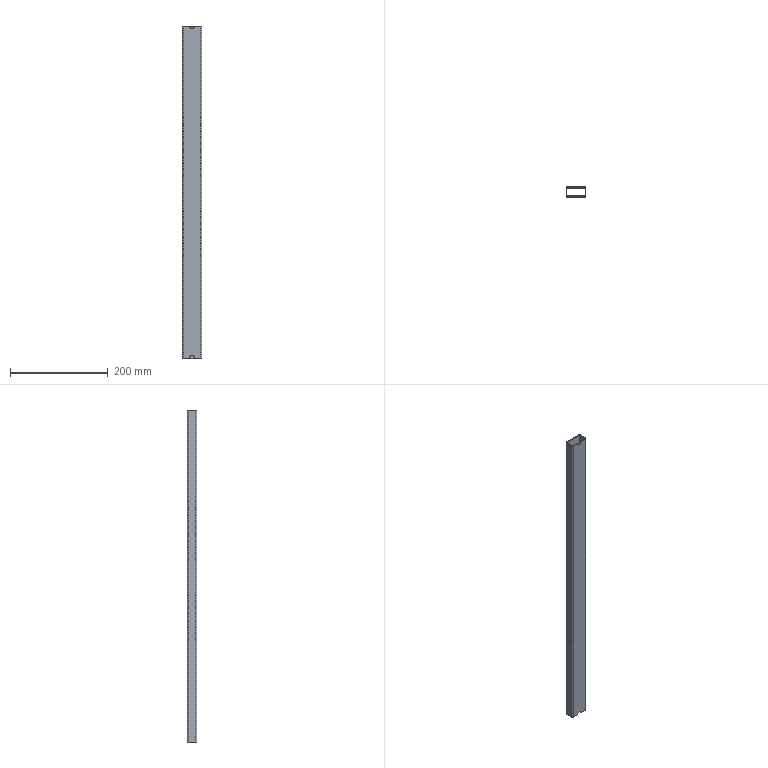Part | STEP file | 6150102 | 1 solid | 20 faces | box 40 x 20 x 680 mm | volume 113098 mm3 | plane 10 | cylinder 10 | commonest cylinder face diameters 2 x4 5 x4 10 x2
STEP:
#1=CARTESIAN_POINT('',(5.,0.,340.));
#2=VERTEX_POINT('',#1);
#3=CARTESIAN_POINT('',(-5.,0.,340.));
#4=VERTEX_POINT('',#3);
#5=CARTESIAN_POINT('',(0.,0.,340.));
#6=DIRECTION('',(0.,1.,0.));
#7=DIRECTION('',(0.,0.,1.));
#8=AXIS2_PLACEMENT_3D('',#5,#6,#7);
#9=CIRCLE('',#8,5.);
#10=EDGE_CURVE('',#2,#4,#9,.T.);
#11=ORIENTED_EDGE('',*,*,#10,.T.);
#12=CARTESIAN_POINT('',(-17.5,0.,340.));
#13=VERTEX_POINT('',#12);
#14=CARTESIAN_POINT('',(17.5,0.,340.));
#15=DIRECTION('',(1.,0.,0.));
#16=VECTOR('',#15,1000.);
#17=LINE('',#14,#16);
#18=EDGE_CURVE('',#13,#4,#17,.T.);
#19=ORIENTED_EDGE('',*,*,#18,.F.);
#20=CARTESIAN_POINT('',(-17.5,0.,-340.));
#21=VERTEX_POINT('',#20);
#22=CARTESIAN_POINT('',(-17.5,0.,340.));
#23=DIRECTION('',(0.,0.,-1.));
#24=VECTOR('',#23,1000.);
#25=LINE('',#22,#24);
#26=EDGE_CURVE('',#13,#21,#25,.T.);
#27=ORIENTED_EDGE('',*,*,#26,.T.);
#28=CARTESIAN_POINT('',(-5.,0.,-340.));
#29=VERTEX_POINT('',#28);
#30=CARTESIAN_POINT('',(17.5,0.,-340.));
#31=DIRECTION('',(1.,0.,0.));
#32=VECTOR('',#31,1000.);
#33=LINE('',#30,#32);
#34=EDGE_CURVE('',#21,#29,#33,.T.);
#35=ORIENTED_EDGE('',*,*,#34,.T.);
#36=CARTESIAN_POINT('',(5.,0.,-340.));
#37=VERTEX_POINT('',#36);
#38=CARTESIAN_POINT('',(0.,0.,-340.));
#39=DIRECTION('',(0.,1.,0.));
#40=DIRECTION('',(0.,0.,1.));
#41=AXIS2_PLACEMENT_3D('',#38,#39,#40);
#42=CIRCLE('',#41,5.);
#43=EDGE_CURVE('',#29,#37,#42,.T.);
#44=ORIENTED_EDGE('',*,*,#43,.T.);
#45=CARTESIAN_POINT('',(17.5,0.,-340.));
#46=VERTEX_POINT('',#45);
#47=CARTESIAN_POINT('',(17.5,0.,-340.));
#48=DIRECTION('',(1.,0.,0.));
#49=VECTOR('',#48,1000.);
#50=LINE('',#47,#49);
#51=EDGE_CURVE('',#37,#46,#50,.T.);
#52=ORIENTED_EDGE('',*,*,#51,.T.);
#53=CARTESIAN_POINT('',(17.5,0.,340.));
#54=VERTEX_POINT('',#53);
#55=CARTESIAN_POINT('',(17.5,0.,340.));
#56=DIRECTION('',(0.,0.,-1.));
#57=VECTOR('',#56,1000.);
#58=LINE('',#55,#57);
#59=EDGE_CURVE('',#54,#46,#58,.T.);
#60=ORIENTED_EDGE('',*,*,#59,.F.);
#61=CARTESIAN_POINT('',(17.5,0.,340.));
#62=DIRECTION('',(1.,0.,0.));
#63=VECTOR('',#62,1000.);
#64=LINE('',#61,#63);
#65=EDGE_CURVE('',#2,#54,#64,.T.);
#66=ORIENTED_EDGE('',*,*,#65,.F.);
#67=EDGE_LOOP('',(#11,#19,#27,#35,#44,#52,#60,#66));
#68=FACE_OUTER_BOUND('',#67,.T.);
#69=CARTESIAN_POINT('',(17.5,0.,340.));
#70=DIRECTION('',(0.,1.,0.));
#71=DIRECTION('',(0.,0.,1.));
#72=AXIS2_PLACEMENT_3D('',#69,#70,#71);
#73=PLANE('',#72);
#74=ADVANCED_FACE('',(#68),#73,.F.);
#75=CARTESIAN_POINT('',(-17.5,1.5,340.));
#76=VERTEX_POINT('',#75);
#77=CARTESIAN_POINT('',(-5.,1.5,340.));
#78=VERTEX_POINT('',#77);
#79=CARTESIAN_POINT('',(17.5,1.5,340.));
#80=DIRECTION('',(1.,0.,0.));
#81=VECTOR('',#80,1000.);
#82=LINE('',#79,#81);
#83=EDGE_CURVE('',#76,#78,#82,.T.);
#84=ORIENTED_EDGE('',*,*,#83,.T.);
#85=CARTESIAN_POINT('',(5.,1.5,340.));
#86=VERTEX_POINT('',#85);
#87=CARTESIAN_POINT('',(0.,1.5,340.));
#88=DIRECTION('',(0.,-1.,0.));
#89=DIRECTION('',(-1.,0.,0.));
#90=AXIS2_PLACEMENT_3D('',#87,#88,#89);
#91=CIRCLE('',#90,5.);
#92=EDGE_CURVE('',#78,#86,#91,.T.);
#93=ORIENTED_EDGE('',*,*,#92,.T.);
#94=CARTESIAN_POINT('',(17.5,1.5,340.));
#95=VERTEX_POINT('',#94);
#96=CARTESIAN_POINT('',(17.5,1.5,340.));
#97=DIRECTION('',(1.,0.,0.));
#98=VECTOR('',#97,1000.);
#99=LINE('',#96,#98);
#100=EDGE_CURVE('',#86,#95,#99,.T.);
#101=ORIENTED_EDGE('',*,*,#100,.T.);
#102=CARTESIAN_POINT('',(17.5,1.5,-340.));
#103=VERTEX_POINT('',#102);
#104=CARTESIAN_POINT('',(17.5,1.5,340.));
#105=DIRECTION('',(0.,0.,-1.));
#106=VECTOR('',#105,1000.);
#107=LINE('',#104,#106);
#108=EDGE_CURVE('',#95,#103,#107,.T.);
#109=ORIENTED_EDGE('',*,*,#108,.T.);
#110=CARTESIAN_POINT('',(5.,1.5,-340.));
#111=VERTEX_POINT('',#110);
#112=CARTESIAN_POINT('',(17.5,1.5,-340.));
#113=DIRECTION('',(1.,0.,0.));
#114=VECTOR('',#113,1000.);
#115=LINE('',#112,#114);
#116=EDGE_CURVE('',#111,#103,#115,.T.);
#117=ORIENTED_EDGE('',*,*,#116,.F.);
#118=CARTESIAN_POINT('',(-5.,1.5,-340.));
#119=VERTEX_POINT('',#118);
#120=CARTESIAN_POINT('',(0.,1.5,-340.));
#121=DIRECTION('',(0.,-1.,0.));
#122=DIRECTION('',(-1.,0.,0.));
#123=AXIS2_PLACEMENT_3D('',#120,#121,#122);
#124=CIRCLE('',#123,5.);
#125=EDGE_CURVE('',#111,#119,#124,.T.);
#126=ORIENTED_EDGE('',*,*,#125,.T.);
#127=CARTESIAN_POINT('',(-17.5,1.5,-340.));
#128=VERTEX_POINT('',#127);
#129=CARTESIAN_POINT('',(17.5,1.5,-340.));
#130=DIRECTION('',(1.,0.,0.));
#131=VECTOR('',#130,1000.);
#132=LINE('',#129,#131);
#133=EDGE_CURVE('',#128,#119,#132,.T.);
#134=ORIENTED_EDGE('',*,*,#133,.F.);
#135=CARTESIAN_POINT('',(-17.5,1.5,340.));
#136=DIRECTION('',(0.,0.,-1.));
#137=VECTOR('',#136,1000.);
#138=LINE('',#135,#137);
#139=EDGE_CURVE('',#76,#128,#138,.T.);
#140=ORIENTED_EDGE('',*,*,#139,.F.);
#141=EDGE_LOOP('',(#84,#93,#101,#109,#117,#126,#134,#140));
#142=FACE_OUTER_BOUND('',#141,.T.);
#143=CARTESIAN_POINT('',(17.5,1.5,340.));
#144=DIRECTION('',(0.,1.,0.));
#145=DIRECTION('',(-1.,0.,0.));
#146=AXIS2_PLACEMENT_3D('',#143,#144,#145);
#147=PLANE('',#146);
#148=ADVANCED_FACE('',(#142),#147,.T.);
#149=CARTESIAN_POINT('',(5.,10.,340.));
#150=DIRECTION('',(0.,1.,0.));
#151=VECTOR('',#150,1000.);
#152=LINE('',#149,#151);
#153=EDGE_CURVE('',#2,#86,#152,.T.);
#154=ORIENTED_EDGE('',*,*,#153,.F.);
#155=ORIENTED_EDGE('',*,*,#65,.T.);
#156=CARTESIAN_POINT('',(20.,2.5,340.));
#157=VERTEX_POINT('',#156);
#158=CARTESIAN_POINT('',(17.5,2.5,340.));
#159=DIRECTION('',(0.,0.,1.));
#160=DIRECTION('',(-1.,0.,0.));
#161=AXIS2_PLACEMENT_3D('',#158,#159,#160);
#162=CIRCLE('',#161,2.5);
#163=EDGE_CURVE('',#54,#157,#162,.T.);
#164=ORIENTED_EDGE('',*,*,#163,.T.);
#165=CARTESIAN_POINT('',(20.,17.5,340.));
#166=VERTEX_POINT('',#165);
#167=CARTESIAN_POINT('',(20.,2.5,340.));
#168=DIRECTION('',(0.,1.,0.));
#169=VECTOR('',#168,1000.);
#170=LINE('',#167,#169);
#171=EDGE_CURVE('',#157,#166,#170,.T.);
#172=ORIENTED_EDGE('',*,*,#171,.T.);
#173=CARTESIAN_POINT('',(17.5,20.,340.));
#174=VERTEX_POINT('',#173);
#175=CARTESIAN_POINT('',(17.5,17.5,340.));
#176=DIRECTION('',(0.,0.,1.));
#177=DIRECTION('',(-1.,0.,0.));
#178=AXIS2_PLACEMENT_3D('',#175,#176,#177);
#179=CIRCLE('',#178,2.5);
#180=EDGE_CURVE('',#166,#174,#179,.T.);
#181=ORIENTED_EDGE('',*,*,#180,.T.);
#182=CARTESIAN_POINT('',(-17.5,20.,340.));
#183=VERTEX_POINT('',#182);
#184=CARTESIAN_POINT('',(17.5,20.,340.));
#185=DIRECTION('',(-1.,0.,0.));
#186=VECTOR('',#185,1000.);
#187=LINE('',#184,#186);
#188=EDGE_CURVE('',#174,#183,#187,.T.);
#189=ORIENTED_EDGE('',*,*,#188,.T.);
#190=CARTESIAN_POINT('',(-20.,17.5,340.));
#191=VERTEX_POINT('',#190);
#192=CARTESIAN_POINT('',(-17.5,17.5,340.));
#193=DIRECTION('',(0.,0.,1.));
#194=DIRECTION('',(-1.,0.,0.));
#195=AXIS2_PLACEMENT_3D('',#192,#193,#194);
#196=CIRCLE('',#195,2.5);
#197=EDGE_CURVE('',#183,#191,#196,.T.);
#198=ORIENTED_EDGE('',*,*,#197,.T.);
#199=CARTESIAN_POINT('',(-20.,2.5,340.));
#200=VERTEX_POINT('',#199);
#201=CARTESIAN_POINT('',(-20.,2.5,340.));
#202=DIRECTION('',(0.,-1.,0.));
#203=VECTOR('',#202,1000.);
#204=LINE('',#201,#203);
#205=EDGE_CURVE('',#191,#200,#204,.T.);
#206=ORIENTED_EDGE('',*,*,#205,.T.);
#207=CARTESIAN_POINT('',(-17.5,2.5,340.));
#208=DIRECTION('',(0.,0.,1.));
#209=DIRECTION('',(-1.,0.,0.));
#210=AXIS2_PLACEMENT_3D('',#207,#208,#209);
#211=CIRCLE('',#210,2.5);
#212=EDGE_CURVE('',#200,#13,#211,.T.);
#213=ORIENTED_EDGE('',*,*,#212,.T.);
#214=ORIENTED_EDGE('',*,*,#18,.T.);
#215=CARTESIAN_POINT('',(-5.,10.,340.));
#216=DIRECTION('',(0.,-1.,0.));
#217=VECTOR('',#216,1000.);
#218=LINE('',#215,#217);
#219=EDGE_CURVE('',#78,#4,#218,.T.);
#220=ORIENTED_EDGE('',*,*,#219,.F.);
#221=ORIENTED_EDGE('',*,*,#83,.F.);
#222=CARTESIAN_POINT('',(-18.5,2.5,340.));
#223=VERTEX_POINT('',#222);
#224=CARTESIAN_POINT('',(-17.5,2.5,340.));
#225=DIRECTION('',(0.,0.,1.));
#226=DIRECTION('',(-1.,0.,0.));
#227=AXIS2_PLACEMENT_3D('',#224,#225,#226);
#228=CIRCLE('',#227,1.);
#229=EDGE_CURVE('',#223,#76,#228,.T.);
#230=ORIENTED_EDGE('',*,*,#229,.F.);
#231=CARTESIAN_POINT('',(-18.5,17.5,340.));
#232=VERTEX_POINT('',#231);
#233=CARTESIAN_POINT('',(-18.5,2.5,340.));
#234=DIRECTION('',(0.,-1.,0.));
#235=VECTOR('',#234,1000.);
#236=LINE('',#233,#235);
#237=EDGE_CURVE('',#232,#223,#236,.T.);
#238=ORIENTED_EDGE('',*,*,#237,.F.);
#239=CARTESIAN_POINT('',(-17.5,18.5,340.));
#240=VERTEX_POINT('',#239);
#241=CARTESIAN_POINT('',(-17.5,17.5,340.));
#242=DIRECTION('',(0.,0.,1.));
#243=DIRECTION('',(-1.,0.,0.));
#244=AXIS2_PLACEMENT_3D('',#241,#242,#243);
#245=CIRCLE('',#244,1.);
#246=EDGE_CURVE('',#240,#232,#245,.T.);
#247=ORIENTED_EDGE('',*,*,#246,.F.);
#248=CARTESIAN_POINT('',(17.5,18.5,340.));
#249=VERTEX_POINT('',#248);
#250=CARTESIAN_POINT('',(17.5,18.5,340.));
#251=DIRECTION('',(-1.,0.,0.));
#252=VECTOR('',#251,1000.);
#253=LINE('',#250,#252);
#254=EDGE_CURVE('',#249,#240,#253,.T.);
#255=ORIENTED_EDGE('',*,*,#254,.F.);
#256=CARTESIAN_POINT('',(18.5,17.5,340.));
#257=VERTEX_POINT('',#256);
#258=CARTESIAN_POINT('',(17.5,17.5,340.));
#259=DIRECTION('',(0.,0.,1.));
#260=DIRECTION('',(-1.,0.,0.));
#261=AXIS2_PLACEMENT_3D('',#258,#259,#260);
#262=CIRCLE('',#261,1.);
#263=EDGE_CURVE('',#257,#249,#262,.T.);
#264=ORIENTED_EDGE('',*,*,#263,.F.);
#265=CARTESIAN_POINT('',(18.5,2.5,340.));
#266=VERTEX_POINT('',#265);
#267=CARTESIAN_POINT('',(18.5,2.5,340.));
#268=DIRECTION('',(0.,1.,0.));
#269=VECTOR('',#268,1000.);
#270=LINE('',#267,#269);
#271=EDGE_CURVE('',#266,#257,#270,.T.);
#272=ORIENTED_EDGE('',*,*,#271,.F.);
#273=CARTESIAN_POINT('',(17.5,2.5,340.));
#274=DIRECTION('',(0.,0.,1.));
#275=DIRECTION('',(-1.,0.,0.));
#276=AXIS2_PLACEMENT_3D('',#273,#274,#275);
#277=CIRCLE('',#276,1.);
#278=EDGE_CURVE('',#95,#266,#277,.T.);
#279=ORIENTED_EDGE('',*,*,#278,.F.);
#280=ORIENTED_EDGE('',*,*,#100,.F.);
#281=EDGE_LOOP('',(#154,#155,#164,#172,#181,#189,#198,#206,#213,#214,#220,#221,#230,#238,#247,#255,#264,#272,#279,#280));
#282=FACE_OUTER_BOUND('',#281,.T.);
#283=CARTESIAN_POINT('',(-17.5,17.5,340.));
#284=DIRECTION('',(0.,0.,-1.));
#285=DIRECTION('',(-1.,0.,0.));
#286=AXIS2_PLACEMENT_3D('',#283,#284,#285);
#287=PLANE('',#286);
#288=ADVANCED_FACE('',(#282),#287,.F.);
#289=ORIENTED_EDGE('',*,*,#51,.F.);
#290=CARTESIAN_POINT('',(5.,10.,-340.));
#291=DIRECTION('',(0.,1.,0.));
#292=VECTOR('',#291,1000.);
#293=LINE('',#290,#292);
#294=EDGE_CURVE('',#37,#111,#293,.T.);
#295=ORIENTED_EDGE('',*,*,#294,.T.);
#296=ORIENTED_EDGE('',*,*,#116,.T.);
#297=CARTESIAN_POINT('',(18.5,2.5,-340.));
#298=VERTEX_POINT('',#297);
#299=CARTESIAN_POINT('',(17.5,2.5,-340.));
#300=DIRECTION('',(0.,0.,1.));
#301=DIRECTION('',(-1.,0.,0.));
#302=AXIS2_PLACEMENT_3D('',#299,#300,#301);
#303=CIRCLE('',#302,1.);
#304=EDGE_CURVE('',#103,#298,#303,.T.);
#305=ORIENTED_EDGE('',*,*,#304,.T.);
#306=CARTESIAN_POINT('',(18.5,17.5,-340.));
#307=VERTEX_POINT('',#306);
#308=CARTESIAN_POINT('',(18.5,2.5,-340.));
#309=DIRECTION('',(0.,1.,0.));
#310=VECTOR('',#309,1000.);
#311=LINE('',#308,#310);
#312=EDGE_CURVE('',#298,#307,#311,.T.);
#313=ORIENTED_EDGE('',*,*,#312,.T.);
#314=CARTESIAN_POINT('',(17.5,18.5,-340.));
#315=VERTEX_POINT('',#314);
#316=CARTESIAN_POINT('',(17.5,17.5,-340.));
#317=DIRECTION('',(0.,0.,1.));
#318=DIRECTION('',(-1.,0.,0.));
#319=AXIS2_PLACEMENT_3D('',#316,#317,#318);
#320=CIRCLE('',#319,1.);
#321=EDGE_CURVE('',#307,#315,#320,.T.);
#322=ORIENTED_EDGE('',*,*,#321,.T.);
#323=CARTESIAN_POINT('',(-17.5,18.5,-340.));
#324=VERTEX_POINT('',#323);
#325=CARTESIAN_POINT('',(17.5,18.5,-340.));
#326=DIRECTION('',(-1.,0.,0.));
#327=VECTOR('',#326,1000.);
#328=LINE('',#325,#327);
#329=EDGE_CURVE('',#315,#324,#328,.T.);
#330=ORIENTED_EDGE('',*,*,#329,.T.);
#331=CARTESIAN_POINT('',(-18.5,17.5,-340.));
#332=VERTEX_POINT('',#331);
#333=CARTESIAN_POINT('',(-17.5,17.5,-340.));
#334=DIRECTION('',(0.,0.,1.));
#335=DIRECTION('',(-1.,0.,0.));
#336=AXIS2_PLACEMENT_3D('',#333,#334,#335);
#337=CIRCLE('',#336,1.);
#338=EDGE_CURVE('',#324,#332,#337,.T.);
#339=ORIENTED_EDGE('',*,*,#338,.T.);
#340=CARTESIAN_POINT('',(-18.5,2.5,-340.));
#341=VERTEX_POINT('',#340);
#342=CARTESIAN_POINT('',(-18.5,2.5,-340.));
#343=DIRECTION('',(0.,-1.,0.));
#344=VECTOR('',#343,1000.);
#345=LINE('',#342,#344);
#346=EDGE_CURVE('',#332,#341,#345,.T.);
#347=ORIENTED_EDGE('',*,*,#346,.T.);
#348=CARTESIAN_POINT('',(-17.5,2.5,-340.));
#349=DIRECTION('',(0.,0.,1.));
#350=DIRECTION('',(-1.,0.,0.));
#351=AXIS2_PLACEMENT_3D('',#348,#349,#350);
#352=CIRCLE('',#351,1.);
#353=EDGE_CURVE('',#341,#128,#352,.T.);
#354=ORIENTED_EDGE('',*,*,#353,.T.);
#355=ORIENTED_EDGE('',*,*,#133,.T.);
#356=CARTESIAN_POINT('',(-5.,10.,-340.));
#357=DIRECTION('',(0.,-1.,0.));
#358=VECTOR('',#357,1000.);
#359=LINE('',#356,#358);
#360=EDGE_CURVE('',#119,#29,#359,.T.);
#361=ORIENTED_EDGE('',*,*,#360,.T.);
#362=ORIENTED_EDGE('',*,*,#34,.F.);
#363=CARTESIAN_POINT('',(-20.,2.5,-340.));
#364=VERTEX_POINT('',#363);
#365=CARTESIAN_POINT('',(-17.5,2.5,-340.));
#366=DIRECTION('',(0.,0.,1.));
#367=DIRECTION('',(-1.,0.,0.));
#368=AXIS2_PLACEMENT_3D('',#365,#366,#367);
#369=CIRCLE('',#368,2.5);
#370=EDGE_CURVE('',#364,#21,#369,.T.);
#371=ORIENTED_EDGE('',*,*,#370,.F.);
#372=CARTESIAN_POINT('',(-20.,17.5,-340.));
#373=VERTEX_POINT('',#372);
#374=CARTESIAN_POINT('',(-20.,2.5,-340.));
#375=DIRECTION('',(0.,-1.,0.));
#376=VECTOR('',#375,1000.);
#377=LINE('',#374,#376);
#378=EDGE_CURVE('',#373,#364,#377,.T.);
#379=ORIENTED_EDGE('',*,*,#378,.F.);
#380=CARTESIAN_POINT('',(-17.5,20.,-340.));
#381=VERTEX_POINT('',#380);
#382=CARTESIAN_POINT('',(-17.5,17.5,-340.));
#383=DIRECTION('',(0.,0.,1.));
#384=DIRECTION('',(-1.,0.,0.));
#385=AXIS2_PLACEMENT_3D('',#382,#383,#384);
#386=CIRCLE('',#385,2.5);
#387=EDGE_CURVE('',#381,#373,#386,.T.);
#388=ORIENTED_EDGE('',*,*,#387,.F.);
#389=CARTESIAN_POINT('',(17.5,20.,-340.));
#390=VERTEX_POINT('',#389);
#391=CARTESIAN_POINT('',(17.5,20.,-340.));
#392=DIRECTION('',(-1.,0.,0.));
#393=VECTOR('',#392,1000.);
#394=LINE('',#391,#393);
#395=EDGE_CURVE('',#390,#381,#394,.T.);
#396=ORIENTED_EDGE('',*,*,#395,.F.);
#397=CARTESIAN_POINT('',(20.,17.5,-340.));
#398=VERTEX_POINT('',#397);
#399=CARTESIAN_POINT('',(17.5,17.5,-340.));
#400=DIRECTION('',(0.,0.,1.));
#401=DIRECTION('',(-1.,0.,0.));
#402=AXIS2_PLACEMENT_3D('',#399,#400,#401);
#403=CIRCLE('',#402,2.5);
#404=EDGE_CURVE('',#398,#390,#403,.T.);
#405=ORIENTED_EDGE('',*,*,#404,.F.);
#406=CARTESIAN_POINT('',(20.,2.5,-340.));
#407=VERTEX_POINT('',#406);
#408=CARTESIAN_POINT('',(20.,2.5,-340.));
#409=DIRECTION('',(0.,1.,0.));
#410=VECTOR('',#409,1000.);
#411=LINE('',#408,#410);
#412=EDGE_CURVE('',#407,#398,#411,.T.);
#413=ORIENTED_EDGE('',*,*,#412,.F.);
#414=CARTESIAN_POINT('',(17.5,2.5,-340.));
#415=DIRECTION('',(0.,0.,1.));
#416=DIRECTION('',(-1.,0.,0.));
#417=AXIS2_PLACEMENT_3D('',#414,#415,#416);
#418=CIRCLE('',#417,2.5);
#419=EDGE_CURVE('',#46,#407,#418,.T.);
#420=ORIENTED_EDGE('',*,*,#419,.F.);
#421=EDGE_LOOP('',(#289,#295,#296,#305,#313,#322,#330,#339,#347,#354,#355,#361,#362,#371,#379,#388,#396,#405,#413,#420));
#422=FACE_OUTER_BOUND('',#421,.T.);
#423=CARTESIAN_POINT('',(-17.5,17.5,-340.));
#424=DIRECTION('',(0.,0.,-1.));
#425=DIRECTION('',(-1.,0.,0.));
#426=AXIS2_PLACEMENT_3D('',#423,#424,#425);
#427=PLANE('',#426);
#428=ADVANCED_FACE('',(#422),#427,.T.);
#429=ORIENTED_EDGE('',*,*,#387,.T.);
#430=CARTESIAN_POINT('',(-20.,17.5,340.));
#431=DIRECTION('',(0.,0.,-1.));
#432=VECTOR('',#431,1000.);
#433=LINE('',#430,#432);
#434=EDGE_CURVE('',#191,#373,#433,.T.);
#435=ORIENTED_EDGE('',*,*,#434,.F.);
#436=ORIENTED_EDGE('',*,*,#197,.F.);
#437=CARTESIAN_POINT('',(-17.5,20.,340.));
#438=DIRECTION('',(0.,0.,-1.));
#439=VECTOR('',#438,1000.);
#440=LINE('',#437,#439);
#441=EDGE_CURVE('',#183,#381,#440,.T.);
#442=ORIENTED_EDGE('',*,*,#441,.T.);
#443=EDGE_LOOP('',(#429,#435,#436,#442));
#444=FACE_OUTER_BOUND('',#443,.T.);
#445=CARTESIAN_POINT('',(-17.5,17.5,340.));
#446=DIRECTION('',(0.,0.,-1.));
#447=DIRECTION('',(-1.,0.,0.));
#448=AXIS2_PLACEMENT_3D('',#445,#446,#447);
#449=CYLINDRICAL_SURFACE('',#448,2.5);
#450=ADVANCED_FACE('',(#444),#449,.T.);
#451=ORIENTED_EDGE('',*,*,#378,.T.);
#452=CARTESIAN_POINT('',(-20.,2.5,340.));
#453=DIRECTION('',(0.,0.,-1.));
#454=VECTOR('',#453,1000.);
#455=LINE('',#452,#454);
#456=EDGE_CURVE('',#200,#364,#455,.T.);
#457=ORIENTED_EDGE('',*,*,#456,.F.);
#458=ORIENTED_EDGE('',*,*,#205,.F.);
#459=ORIENTED_EDGE('',*,*,#434,.T.);
#460=EDGE_LOOP('',(#451,#457,#458,#459));
#461=FACE_OUTER_BOUND('',#460,.T.);
#462=CARTESIAN_POINT('',(-20.,2.5,340.));
#463=DIRECTION('',(1.,0.,0.));
#464=DIRECTION('',(0.,1.,0.));
#465=AXIS2_PLACEMENT_3D('',#462,#463,#464);
#466=PLANE('',#465);
#467=ADVANCED_FACE('',(#461),#466,.F.);
#468=ORIENTED_EDGE('',*,*,#370,.T.);
#469=ORIENTED_EDGE('',*,*,#26,.F.);
#470=ORIENTED_EDGE('',*,*,#212,.F.);
#471=ORIENTED_EDGE('',*,*,#456,.T.);
#472=EDGE_LOOP('',(#468,#469,#470,#471));
#473=FACE_OUTER_BOUND('',#472,.T.);
#474=CARTESIAN_POINT('',(-17.5,2.5,340.));
#475=DIRECTION('',(0.,0.,-1.));
#476=DIRECTION('',(-1.,0.,0.));
#477=AXIS2_PLACEMENT_3D('',#474,#475,#476);
#478=CYLINDRICAL_SURFACE('',#477,2.5);
#479=ADVANCED_FACE('',(#473),#478,.T.);
#480=ORIENTED_EDGE('',*,*,#419,.T.);
#481=CARTESIAN_POINT('',(20.,2.5,340.));
#482=DIRECTION('',(0.,0.,-1.));
#483=VECTOR('',#482,1000.);
#484=LINE('',#481,#483);
#485=EDGE_CURVE('',#157,#407,#484,.T.);
#486=ORIENTED_EDGE('',*,*,#485,.F.);
#487=ORIENTED_EDGE('',*,*,#163,.F.);
#488=ORIENTED_EDGE('',*,*,#59,.T.);
#489=EDGE_LOOP('',(#480,#486,#487,#488));
#490=FACE_OUTER_BOUND('',#489,.T.);
#491=CARTESIAN_POINT('',(17.5,2.5,340.));
#492=DIRECTION('',(0.,0.,-1.));
#493=DIRECTION('',(-1.,0.,0.));
#494=AXIS2_PLACEMENT_3D('',#491,#492,#493);
#495=CYLINDRICAL_SURFACE('',#494,2.5);
#496=ADVANCED_FACE('',(#490),#495,.T.);
#497=ORIENTED_EDGE('',*,*,#412,.T.);
#498=CARTESIAN_POINT('',(20.,17.5,340.));
#499=DIRECTION('',(0.,0.,-1.));
#500=VECTOR('',#499,1000.);
#501=LINE('',#498,#500);
#502=EDGE_CURVE('',#166,#398,#501,.T.);
#503=ORIENTED_EDGE('',*,*,#502,.F.);
#504=ORIENTED_EDGE('',*,*,#171,.F.);
#505=ORIENTED_EDGE('',*,*,#485,.T.);
#506=EDGE_LOOP('',(#497,#503,#504,#505));
#507=FACE_OUTER_BOUND('',#506,.T.);
#508=CARTESIAN_POINT('',(20.,2.5,340.));
#509=DIRECTION('',(-1.,0.,0.));
#510=DIRECTION('',(0.,-1.,0.));
#511=AXIS2_PLACEMENT_3D('',#508,#509,#510);
#512=PLANE('',#511);
#513=ADVANCED_FACE('',(#507),#512,.F.);
#514=ORIENTED_EDGE('',*,*,#404,.T.);
#515=CARTESIAN_POINT('',(17.5,20.,340.));
#516=DIRECTION('',(0.,0.,-1.));
#517=VECTOR('',#516,1000.);
#518=LINE('',#515,#517);
#519=EDGE_CURVE('',#174,#390,#518,.T.);
#520=ORIENTED_EDGE('',*,*,#519,.F.);
#521=ORIENTED_EDGE('',*,*,#180,.F.);
#522=ORIENTED_EDGE('',*,*,#502,.T.);
#523=EDGE_LOOP('',(#514,#520,#521,#522));
#524=FACE_OUTER_BOUND('',#523,.T.);
#525=CARTESIAN_POINT('',(17.5,17.5,340.));
#526=DIRECTION('',(0.,0.,-1.));
#527=DIRECTION('',(-1.,0.,0.));
#528=AXIS2_PLACEMENT_3D('',#525,#526,#527);
#529=CYLINDRICAL_SURFACE('',#528,2.5);
#530=ADVANCED_FACE('',(#524),#529,.T.);
#531=ORIENTED_EDGE('',*,*,#395,.T.);
#532=ORIENTED_EDGE('',*,*,#441,.F.);
#533=ORIENTED_EDGE('',*,*,#188,.F.);
#534=ORIENTED_EDGE('',*,*,#519,.T.);
#535=EDGE_LOOP('',(#531,#532,#533,#534));
#536=FACE_OUTER_BOUND('',#535,.T.);
#537=CARTESIAN_POINT('',(17.5,20.,340.));
#538=DIRECTION('',(0.,-1.,0.));
#539=DIRECTION('',(0.,0.,-1.));
#540=AXIS2_PLACEMENT_3D('',#537,#538,#539);
#541=PLANE('',#540);
#542=ADVANCED_FACE('',(#536),#541,.F.);
#543=ORIENTED_EDGE('',*,*,#304,.F.);
#544=ORIENTED_EDGE('',*,*,#108,.F.);
#545=ORIENTED_EDGE('',*,*,#278,.T.);
#546=CARTESIAN_POINT('',(18.5,2.5,340.));
#547=DIRECTION('',(0.,0.,-1.));
#548=VECTOR('',#547,1000.);
#549=LINE('',#546,#548);
#550=EDGE_CURVE('',#266,#298,#549,.T.);
#551=ORIENTED_EDGE('',*,*,#550,.T.);
#552=EDGE_LOOP('',(#543,#544,#545,#551));
#553=FACE_OUTER_BOUND('',#552,.T.);
#554=CARTESIAN_POINT('',(17.5,2.5,340.));
#555=DIRECTION('',(0.,0.,-1.));
#556=DIRECTION('',(-1.,0.,0.));
#557=AXIS2_PLACEMENT_3D('',#554,#555,#556);
#558=CYLINDRICAL_SURFACE('',#557,1.);
#559=ADVANCED_FACE('',(#553),#558,.F.);
#560=ORIENTED_EDGE('',*,*,#312,.F.);
#561=ORIENTED_EDGE('',*,*,#550,.F.);
#562=ORIENTED_EDGE('',*,*,#271,.T.);
#563=CARTESIAN_POINT('',(18.5,17.5,340.));
#564=DIRECTION('',(0.,0.,-1.));
#565=VECTOR('',#564,1000.);
#566=LINE('',#563,#565);
#567=EDGE_CURVE('',#257,#307,#566,.T.);
#568=ORIENTED_EDGE('',*,*,#567,.T.);
#569=EDGE_LOOP('',(#560,#561,#562,#568));
#570=FACE_OUTER_BOUND('',#569,.T.);
#571=CARTESIAN_POINT('',(18.5,2.5,340.));
#572=DIRECTION('',(-1.,0.,0.));
#573=DIRECTION('',(0.,-1.,0.));
#574=AXIS2_PLACEMENT_3D('',#571,#572,#573);
#575=PLANE('',#574);
#576=ADVANCED_FACE('',(#570),#575,.T.);
#577=ORIENTED_EDGE('',*,*,#321,.F.);
#578=ORIENTED_EDGE('',*,*,#567,.F.);
#579=ORIENTED_EDGE('',*,*,#263,.T.);
#580=CARTESIAN_POINT('',(17.5,18.5,340.));
#581=DIRECTION('',(0.,0.,-1.));
#582=VECTOR('',#581,1000.);
#583=LINE('',#580,#582);
#584=EDGE_CURVE('',#249,#315,#583,.T.);
#585=ORIENTED_EDGE('',*,*,#584,.T.);
#586=EDGE_LOOP('',(#577,#578,#579,#585));
#587=FACE_OUTER_BOUND('',#586,.T.);
#588=CARTESIAN_POINT('',(17.5,17.5,340.));
#589=DIRECTION('',(0.,0.,-1.));
#590=DIRECTION('',(-1.,0.,0.));
#591=AXIS2_PLACEMENT_3D('',#588,#589,#590);
#592=CYLINDRICAL_SURFACE('',#591,1.);
#593=ADVANCED_FACE('',(#587),#592,.F.);
#594=ORIENTED_EDGE('',*,*,#329,.F.);
#595=ORIENTED_EDGE('',*,*,#584,.F.);
#596=ORIENTED_EDGE('',*,*,#254,.T.);
#597=CARTESIAN_POINT('',(-17.5,18.5,340.));
#598=DIRECTION('',(0.,0.,-1.));
#599=VECTOR('',#598,1000.);
#600=LINE('',#597,#599);
#601=EDGE_CURVE('',#240,#324,#600,.T.);
#602=ORIENTED_EDGE('',*,*,#601,.T.);
#603=EDGE_LOOP('',(#594,#595,#596,#602));
#604=FACE_OUTER_BOUND('',#603,.T.);
#605=CARTESIAN_POINT('',(17.5,18.5,340.));
#606=DIRECTION('',(0.,-1.,0.));
#607=DIRECTION('',(0.,0.,-1.));
#608=AXIS2_PLACEMENT_3D('',#605,#606,#607);
#609=PLANE('',#608);
#610=ADVANCED_FACE('',(#604),#609,.T.);
#611=ORIENTED_EDGE('',*,*,#338,.F.);
#612=ORIENTED_EDGE('',*,*,#601,.F.);
#613=ORIENTED_EDGE('',*,*,#246,.T.);
#614=CARTESIAN_POINT('',(-18.5,17.5,340.));
#615=DIRECTION('',(0.,0.,-1.));
#616=VECTOR('',#615,1000.);
#617=LINE('',#614,#616);
#618=EDGE_CURVE('',#232,#332,#617,.T.);
#619=ORIENTED_EDGE('',*,*,#618,.T.);
#620=EDGE_LOOP('',(#611,#612,#613,#619));
#621=FACE_OUTER_BOUND('',#620,.T.);
#622=CARTESIAN_POINT('',(-17.5,17.5,340.));
#623=DIRECTION('',(0.,0.,-1.));
#624=DIRECTION('',(-1.,0.,0.));
#625=AXIS2_PLACEMENT_3D('',#622,#623,#624);
#626=CYLINDRICAL_SURFACE('',#625,1.);
#627=ADVANCED_FACE('',(#621),#626,.F.);
#628=ORIENTED_EDGE('',*,*,#346,.F.);
#629=ORIENTED_EDGE('',*,*,#618,.F.);
#630=ORIENTED_EDGE('',*,*,#237,.T.);
#631=CARTESIAN_POINT('',(-18.5,2.5,340.));
#632=DIRECTION('',(0.,0.,-1.));
#633=VECTOR('',#632,1000.);
#634=LINE('',#631,#633);
#635=EDGE_CURVE('',#223,#341,#634,.T.);
#636=ORIENTED_EDGE('',*,*,#635,.T.);
#637=EDGE_LOOP('',(#628,#629,#630,#636));
#638=FACE_OUTER_BOUND('',#637,.T.);
#639=CARTESIAN_POINT('',(-18.5,2.5,340.));
#640=DIRECTION('',(1.,0.,0.));
#641=DIRECTION('',(0.,1.,0.));
#642=AXIS2_PLACEMENT_3D('',#639,#640,#641);
#643=PLANE('',#642);
#644=ADVANCED_FACE('',(#638),#643,.T.);
#645=ORIENTED_EDGE('',*,*,#353,.F.);
#646=ORIENTED_EDGE('',*,*,#635,.F.);
#647=ORIENTED_EDGE('',*,*,#229,.T.);
#648=ORIENTED_EDGE('',*,*,#139,.T.);
#649=EDGE_LOOP('',(#645,#646,#647,#648));
#650=FACE_OUTER_BOUND('',#649,.T.);
#651=CARTESIAN_POINT('',(-17.5,2.5,340.));
#652=DIRECTION('',(0.,0.,-1.));
#653=DIRECTION('',(-1.,0.,0.));
#654=AXIS2_PLACEMENT_3D('',#651,#652,#653);
#655=CYLINDRICAL_SURFACE('',#654,1.);
#656=ADVANCED_FACE('',(#650),#655,.F.);
#657=ORIENTED_EDGE('',*,*,#43,.F.);
#658=ORIENTED_EDGE('',*,*,#360,.F.);
#659=ORIENTED_EDGE('',*,*,#125,.F.);
#660=ORIENTED_EDGE('',*,*,#294,.F.);
#661=EDGE_LOOP('',(#657,#658,#659,#660));
#662=FACE_OUTER_BOUND('',#661,.T.);
#663=CARTESIAN_POINT('',(0.,10.,-340.));
#664=DIRECTION('',(0.,-1.,0.));
#665=DIRECTION('',(0.,0.,-1.));
#666=AXIS2_PLACEMENT_3D('',#663,#664,#665);
#667=CYLINDRICAL_SURFACE('',#666,5.);
#668=ADVANCED_FACE('',(#662),#667,.F.);
#669=ORIENTED_EDGE('',*,*,#153,.T.);
#670=ORIENTED_EDGE('',*,*,#92,.F.);
#671=ORIENTED_EDGE('',*,*,#219,.T.);
#672=ORIENTED_EDGE('',*,*,#10,.F.);
#673=EDGE_LOOP('',(#669,#670,#671,#672));
#674=FACE_OUTER_BOUND('',#673,.T.);
#675=CARTESIAN_POINT('',(0.,10.,340.));
#676=DIRECTION('',(0.,-1.,0.));
#677=DIRECTION('',(0.,0.,-1.));
#678=AXIS2_PLACEMENT_3D('',#675,#676,#677);
#679=CYLINDRICAL_SURFACE('',#678,5.);
#680=ADVANCED_FACE('',(#674),#679,.F.);
#681=CLOSED_SHELL('',(#74,#148,#288,#428,#450,#467,#479,#496,#513,#530,#542,#559,#576,#593,#610,#627,#644,#656,#668,#680));
#682=MANIFOLD_SOLID_BREP('',#681);
#683=CARTESIAN_POINT('',(0.,0.,0.));
#684=DIRECTION('',(0.,0.,1.));
#685=DIRECTION('',(1.,0.,0.));
#686=AXIS2_PLACEMENT_3D('',#683,#684,#685);
#687=(LENGTH_UNIT()NAMED_UNIT(*)SI_UNIT(.MILLI.,.METRE.));
#688=UNCERTAINTY_MEASURE_WITH_UNIT(LENGTH_MEASURE(0.00001),#687,'','');
#689=(NAMED_UNIT(*)PLANE_ANGLE_UNIT()SI_UNIT($,.RADIAN.));
#690=(NAMED_UNIT(*)SI_UNIT($,.STERADIAN.)SOLID_ANGLE_UNIT());
#691=(GEOMETRIC_REPRESENTATION_CONTEXT(3)GLOBAL_UNCERTAINTY_ASSIGNED_CONTEXT((#688))GLOBAL_UNIT_ASSIGNED_CONTEXT((#687,#689,#690))REPRESENTATION_CONTEXT('',''));
#692=ADVANCED_BREP_SHAPE_REPRESENTATION('',(#682,#686),#691);